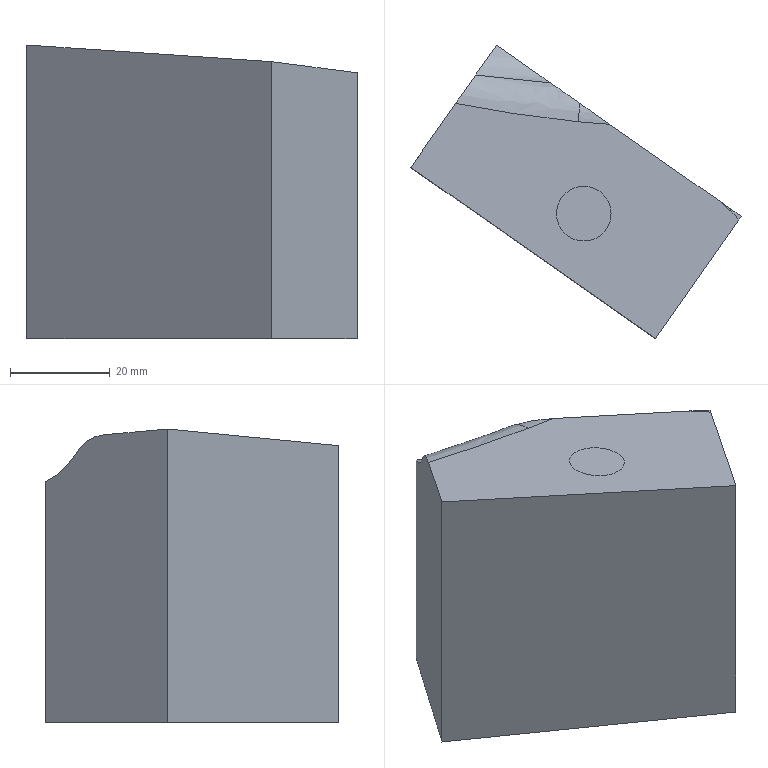Part | NX | features solid 2 | 1 solid | 12 faces | box 66.356 x 58.989 x 59.079 mm | volume 100854 mm3 | spline 7 | plane 5
STEP:
#1=CARTESIAN_POINT('',(-576.236,51.557,-40.));
#2=VERTEX_POINT('',#1);
#3=CARTESIAN_POINT('',(-559.029,76.131,-40.));
#4=VERTEX_POINT('',#3);
#5=CARTESIAN_POINT('',(-576.236,51.557,-40.));
#6=DIRECTION('',(-0.5736,-0.8192,0.));
#7=VECTOR('',#6,1000.);
#8=LINE('',#5,#7);
#9=EDGE_CURVE('',#2,#4,#8,.F.);
#10=ORIENTED_EDGE('',*,*,#9,.F.);
#11=CARTESIAN_POINT('',(-625.385,85.971,-40.));
#12=VERTEX_POINT('',#11);
#13=CARTESIAN_POINT('',(-543.47,28.614,-40.));
#14=DIRECTION('',(-0.8192,0.5736,0.));
#15=VECTOR('',#14,1000.);
#16=LINE('',#13,#15);
#17=EDGE_CURVE('',#12,#2,#16,.F.);
#18=ORIENTED_EDGE('',*,*,#17,.F.);
#19=CARTESIAN_POINT('',(-608.178,110.546,-40.));
#20=VERTEX_POINT('',#19);
#21=CARTESIAN_POINT('',(-625.385,85.971,-40.));
#22=DIRECTION('',(-0.5736,-0.8192,0.));
#23=VECTOR('',#22,1000.);
#24=LINE('',#21,#23);
#25=EDGE_CURVE('',#12,#20,#24,.F.);
#26=ORIENTED_EDGE('',*,*,#25,.T.);
#27=CARTESIAN_POINT('',(-526.263,53.188,-40.));
#28=DIRECTION('',(-0.8192,0.5736,0.));
#29=VECTOR('',#28,1000.);
#30=LINE('',#27,#29);
#31=EDGE_CURVE('',#20,#4,#30,.F.);
#32=ORIENTED_EDGE('',*,*,#31,.T.);
#33=EDGE_LOOP('',(#10,#18,#26,#32));
#34=FACE_BOUND('',#33,.T.);
#35=CARTESIAN_POINT('',(-543.47,28.614,-40.));
#36=DIRECTION('',(0.,0.,1.));
#37=DIRECTION('',(-0.8192,0.5736,0.));
#38=AXIS2_PLACEMENT_3D('',#35,#36,#37);
#39=PLANE('',#38);
#40=ADVANCED_FACE('',(#34),#39,.F.);
#41=CARTESIAN_POINT('',(-563.258,79.093,13.789));
#42=VERTEX_POINT('',#41);
#43=CARTESIAN_POINT('',(-560.662,77.274,13.604));
#44=VERTEX_POINT('',#43);
#45=CARTESIAN_POINT('',(-563.258,79.093,13.789));
#46=CARTESIAN_POINT('',(-562.393,78.487,13.731));
#47=CARTESIAN_POINT('',(-561.527,77.88,13.669));
#48=CARTESIAN_POINT('',(-560.661,77.274,13.604));
#49=B_SPLINE_CURVE_WITH_KNOTS('',3,(#45,#46,#47,#48),.UNSPECIFIED.,.F.,.F.,(4,4),(0.,0.003176),.UNSPECIFIED.);
#50=EDGE_CURVE('',#42,#44,#49,.T.);
#51=ORIENTED_EDGE('',*,*,#50,.T.);
#52=CARTESIAN_POINT('',(-559.029,76.131,13.461));
#53=VERTEX_POINT('',#52);
#54=CARTESIAN_POINT('',(-560.662,77.275,13.604));
#55=CARTESIAN_POINT('',(-560.117,76.893,13.563));
#56=CARTESIAN_POINT('',(-559.573,76.512,13.519));
#57=CARTESIAN_POINT('',(-559.029,76.131,13.461));
#58=B_SPLINE_CURVE_WITH_KNOTS('',3,(#54,#55,#56,#57),.UNSPECIFIED.,.F.,.F.,(4,4),(0.0004081,0.002407),.UNSPECIFIED.);
#59=EDGE_CURVE('',#44,#53,#58,.T.);
#60=ORIENTED_EDGE('',*,*,#59,.T.);
#61=CARTESIAN_POINT('',(-559.029,76.131,80.));
#62=DIRECTION('',(0.,0.,-1.));
#63=VECTOR('',#62,1000.);
#64=LINE('',#61,#63);
#65=EDGE_CURVE('',#53,#4,#64,.T.);
#66=ORIENTED_EDGE('',*,*,#65,.T.);
#67=ORIENTED_EDGE('',*,*,#31,.F.);
#68=CARTESIAN_POINT('',(-608.178,110.546,8.511));
#69=VERTEX_POINT('',#68);
#70=CARTESIAN_POINT('',(-608.178,110.546,80.));
#71=DIRECTION('',(0.,0.,-1.));
#72=VECTOR('',#71,1000.);
#73=LINE('',#70,#72);
#74=EDGE_CURVE('',#69,#20,#73,.T.);
#75=ORIENTED_EDGE('',*,*,#74,.F.);
#76=CARTESIAN_POINT('',(-597.294,102.925,11.329));
#77=VERTEX_POINT('',#76);
#78=CARTESIAN_POINT('',(-608.178,110.546,8.511));
#79=CARTESIAN_POINT('',(-606.271,109.211,8.19));
#80=CARTESIAN_POINT('',(-603.392,107.195,8.072));
#81=CARTESIAN_POINT('',(-599.628,104.559,9.191));
#82=CARTESIAN_POINT('',(-597.942,103.379,10.457));
#83=CARTESIAN_POINT('',(-597.295,102.925,11.328));
#84=B_SPLINE_CURVE_WITH_KNOTS('',3,(#78,#79,#80,#81,#82,#83),.UNSPECIFIED.,.F.,.F.,(4,1,1,4),(0.,0.006983,0.01047,0.01397),.UNSPECIFIED.);
#85=EDGE_CURVE('',#69,#77,#84,.T.);
#86=ORIENTED_EDGE('',*,*,#85,.T.);
#87=CARTESIAN_POINT('',(-591.493,98.863,14.745));
#88=VERTEX_POINT('',#87);
#89=CARTESIAN_POINT('',(-597.294,102.924,11.33));
#90=CARTESIAN_POINT('',(-596.55,102.404,12.332));
#91=CARTESIAN_POINT('',(-594.649,101.073,13.706));
#92=CARTESIAN_POINT('',(-592.562,99.612,14.469));
#93=CARTESIAN_POINT('',(-591.492,98.862,14.745));
#94=B_SPLINE_CURVE_WITH_KNOTS('',3,(#89,#90,#91,#92,#93),.UNSPECIFIED.,.F.,.F.,(4,1,4),(0.,0.00397,0.007939),.UNSPECIFIED.);
#95=EDGE_CURVE('',#77,#88,#94,.T.);
#96=ORIENTED_EDGE('',*,*,#95,.T.);
#97=CARTESIAN_POINT('',(-585.405,94.6,15.297));
#98=VERTEX_POINT('',#97);
#99=CARTESIAN_POINT('',(-585.405,94.6,15.296));
#100=CARTESIAN_POINT('',(-586.428,95.316,15.367));
#101=CARTESIAN_POINT('',(-588.482,96.754,15.411));
#102=CARTESIAN_POINT('',(-590.493,98.163,15.003));
#103=CARTESIAN_POINT('',(-591.495,98.864,14.744));
#104=B_SPLINE_CURVE_WITH_KNOTS('',3,(#99,#100,#101,#102,#103),.UNSPECIFIED.,.F.,.F.,(4,1,4),(0.004974,0.008726,0.01248),.UNSPECIFIED.);
#105=EDGE_CURVE('',#98,#88,#104,.T.);
#106=ORIENTED_EDGE('',*,*,#105,.F.);
#107=CARTESIAN_POINT('',(-611.053,112.559,17.042));
#108=DIRECTION('',(-0.8179,0.5727,0.05566));
#109=VECTOR('',#108,1000.);
#110=LINE('',#107,#109);
#111=EDGE_CURVE('',#98,#42,#110,.F.);
#112=ORIENTED_EDGE('',*,*,#111,.T.);
#113=EDGE_LOOP('',(#51,#60,#66,#67,#75,#86,#96,#106,#112));
#114=FACE_BOUND('',#113,.T.);
#115=CARTESIAN_POINT('',(-608.178,110.546,80.));
#116=DIRECTION('',(0.5736,0.8192,0.));
#117=DIRECTION('',(-0.8192,0.5736,0.));
#118=AXIS2_PLACEMENT_3D('',#115,#116,#117);
#119=PLANE('',#118);
#120=ADVANCED_FACE('',(#114),#119,.T.);
#121=CARTESIAN_POINT('',(-625.385,85.971,19.079));
#122=VERTEX_POINT('',#121);
#123=CARTESIAN_POINT('',(-625.385,85.971,80.));
#124=DIRECTION('',(0.,0.,-1.));
#125=VECTOR('',#124,1000.);
#126=LINE('',#123,#125);
#127=EDGE_CURVE('',#122,#12,#126,.T.);
#128=ORIENTED_EDGE('',*,*,#127,.F.);
#129=CARTESIAN_POINT('',(-616.399,98.804,17.913));
#130=VERTEX_POINT('',#129);
#131=CARTESIAN_POINT('',(-627.971,82.279,19.414));
#132=DIRECTION('',(-0.572,-0.8169,0.0742));
#133=VECTOR('',#132,1000.);
#134=LINE('',#131,#133);
#135=EDGE_CURVE('',#122,#130,#134,.F.);
#136=ORIENTED_EDGE('',*,*,#135,.T.);
#137=CARTESIAN_POINT('',(-612.406,104.507,14.025));
#138=VERTEX_POINT('',#137);
#139=CARTESIAN_POINT('',(-616.399,98.805,17.913));
#140=CARTESIAN_POINT('',(-614.817,101.064,17.708));
#141=CARTESIAN_POINT('',(-613.314,103.21,16.305));
#142=CARTESIAN_POINT('',(-612.408,104.504,14.03));
#143=B_SPLINE_CURVE_WITH_KNOTS('',3,(#139,#140,#141,#142),.UNSPECIFIED.,.F.,.F.,(4,4),(0.,0.008252),.UNSPECIFIED.);
#144=EDGE_CURVE('',#130,#138,#143,.T.);
#145=ORIENTED_EDGE('',*,*,#144,.T.);
#146=CARTESIAN_POINT('',(-612.406,104.508,14.024));
#147=CARTESIAN_POINT('',(-611.379,105.974,11.449));
#148=CARTESIAN_POINT('',(-609.88,108.114,9.542));
#149=CARTESIAN_POINT('',(-608.178,110.546,8.511));
#150=B_SPLINE_CURVE_WITH_KNOTS('',3,(#146,#147,#148,#149),.UNSPECIFIED.,.F.,.F.,(4,4),(0.003915,0.01322),.UNSPECIFIED.);
#151=EDGE_CURVE('',#138,#69,#150,.T.);
#152=ORIENTED_EDGE('',*,*,#151,.T.);
#153=ORIENTED_EDGE('',*,*,#74,.T.);
#154=ORIENTED_EDGE('',*,*,#25,.F.);
#155=EDGE_LOOP('',(#128,#136,#145,#152,#153,#154));
#156=FACE_BOUND('',#155,.T.);
#157=CARTESIAN_POINT('',(-625.385,85.971,80.));
#158=DIRECTION('',(-0.8192,0.5736,0.));
#159=DIRECTION('',(-0.5736,-0.8192,0.));
#160=AXIS2_PLACEMENT_3D('',#157,#158,#159);
#161=PLANE('',#160);
#162=ADVANCED_FACE('',(#156),#161,.T.);
#163=CARTESIAN_POINT('',(-576.236,51.557,15.734));
#164=VERTEX_POINT('',#163);
#165=CARTESIAN_POINT('',(-628.159,87.913,19.267));
#166=DIRECTION('',(-0.8179,0.5727,0.05566));
#167=VECTOR('',#166,1000.);
#168=LINE('',#165,#167);
#169=EDGE_CURVE('',#122,#164,#168,.F.);
#170=ORIENTED_EDGE('',*,*,#169,.F.);
#171=ORIENTED_EDGE('',*,*,#127,.T.);
#172=ORIENTED_EDGE('',*,*,#17,.T.);
#173=CARTESIAN_POINT('',(-576.236,51.557,80.));
#174=DIRECTION('',(0.,0.,-1.));
#175=VECTOR('',#174,1000.);
#176=LINE('',#173,#175);
#177=EDGE_CURVE('',#164,#2,#176,.T.);
#178=ORIENTED_EDGE('',*,*,#177,.F.);
#179=EDGE_LOOP('',(#170,#171,#172,#178));
#180=FACE_BOUND('',#179,.T.);
#181=CARTESIAN_POINT('',(-625.385,85.971,80.));
#182=DIRECTION('',(0.5736,0.8192,0.));
#183=DIRECTION('',(-0.8192,0.5736,0.));
#184=AXIS2_PLACEMENT_3D('',#181,#182,#183);
#185=PLANE('',#184);
#186=ADVANCED_FACE('',(#180),#185,.F.);
#187=CARTESIAN_POINT('',(-559.56,75.373,13.571));
#188=VERTEX_POINT('',#187);
#189=CARTESIAN_POINT('',(-578.964,47.661,16.088));
#190=DIRECTION('',(-0.572,-0.8169,0.0742));
#191=VECTOR('',#190,1000.);
#192=LINE('',#189,#191);
#193=EDGE_CURVE('',#164,#188,#192,.F.);
#194=ORIENTED_EDGE('',*,*,#193,.F.);
#195=ORIENTED_EDGE('',*,*,#177,.T.);
#196=ORIENTED_EDGE('',*,*,#9,.T.);
#197=ORIENTED_EDGE('',*,*,#65,.F.);
#198=CARTESIAN_POINT('',(-559.56,75.373,13.57));
#199=CARTESIAN_POINT('',(-559.383,75.626,13.547));
#200=CARTESIAN_POINT('',(-559.206,75.879,13.512));
#201=CARTESIAN_POINT('',(-559.029,76.131,13.461));
#202=B_SPLINE_CURVE_WITH_KNOTS('',3,(#198,#199,#200,#201),.UNSPECIFIED.,.F.,.F.,(4,4),(0.003283,0.004211),.UNSPECIFIED.);
#203=EDGE_CURVE('',#188,#53,#202,.T.);
#204=ORIENTED_EDGE('',*,*,#203,.F.);
#205=EDGE_LOOP('',(#194,#195,#196,#197,#204));
#206=FACE_BOUND('',#205,.T.);
#207=CARTESIAN_POINT('',(-576.236,51.557,80.));
#208=DIRECTION('',(-0.8192,0.5736,0.));
#209=DIRECTION('',(-0.5736,-0.8192,0.));
#210=AXIS2_PLACEMENT_3D('',#207,#208,#209);
#211=PLANE('',#210);
#212=ADVANCED_FACE('',(#206),#211,.F.);
#213=CARTESIAN_POINT('',(-596.124,76.649,16.764));
#214=VERTEX_POINT('',#213);
#215=CARTESIAN_POINT('',(-585.166,76.649,15.796));
#216=VERTEX_POINT('',#215);
#217=CARTESIAN_POINT('',(-596.124,76.649,16.764));
#218=CARTESIAN_POINT('',(-596.122,75.89,16.785));
#219=CARTESIAN_POINT('',(-595.863,74.494,16.803));
#220=CARTESIAN_POINT('',(-594.599,72.667,16.744));
#221=CARTESIAN_POINT('',(-592.796,71.409,16.621));
#222=CARTESIAN_POINT('',(-590.631,71.023,16.441));
#223=CARTESIAN_POINT('',(-588.469,71.408,16.239));
#224=CARTESIAN_POINT('',(-586.671,72.667,16.044));
#225=CARTESIAN_POINT('',(-585.416,74.494,15.88));
#226=CARTESIAN_POINT('',(-585.165,75.89,15.818));
#227=CARTESIAN_POINT('',(-585.166,76.649,15.796));
#228=B_SPLINE_CURVE_WITH_KNOTS('',3,(#217,#218,#219,#220,#221,#222,#223,#224,#225,#226,#227),.UNSPECIFIED.,.F.,.F.,(4,1,1,1,1,1,1,1,4),(0.,0.125,0.25,0.375,0.5,0.625,0.75,0.875,1.),.UNSPECIFIED.);
#229=EDGE_CURVE('',#214,#216,#228,.T.);
#230=ORIENTED_EDGE('',*,*,#229,.F.);
#231=CARTESIAN_POINT('',(-585.166,76.649,15.796));
#232=CARTESIAN_POINT('',(-585.168,77.408,15.774));
#233=CARTESIAN_POINT('',(-585.427,78.804,15.756));
#234=CARTESIAN_POINT('',(-586.691,80.632,15.815));
#235=CARTESIAN_POINT('',(-588.494,81.89,15.938));
#236=CARTESIAN_POINT('',(-590.66,82.275,16.118));
#237=CARTESIAN_POINT('',(-592.822,81.89,16.32));
#238=CARTESIAN_POINT('',(-594.62,80.631,16.515));
#239=CARTESIAN_POINT('',(-595.874,78.804,16.679));
#240=CARTESIAN_POINT('',(-596.126,77.408,16.742));
#241=CARTESIAN_POINT('',(-596.124,76.649,16.764));
#242=B_SPLINE_CURVE_WITH_KNOTS('',3,(#231,#232,#233,#234,#235,#236,#237,#238,#239,#240,#241),.UNSPECIFIED.,.F.,.F.,(4,1,1,1,1,1,1,1,4),(0.,0.125,0.25,0.375,0.5,0.625,0.75,0.875,1.),.UNSPECIFIED.);
#243=EDGE_CURVE('',#216,#214,#242,.T.);
#244=ORIENTED_EDGE('',*,*,#243,.F.);
#245=EDGE_LOOP('',(#230,#244));
#246=FACE_BOUND('',#245,.T.);
#247=ORIENTED_EDGE('',*,*,#193,.T.);
#248=CARTESIAN_POINT('',(-560.907,76.996,13.642));
#249=VERTEX_POINT('',#248);
#250=CARTESIAN_POINT('',(-560.907,76.996,13.643));
#251=CARTESIAN_POINT('',(-560.377,76.523,13.609));
#252=CARTESIAN_POINT('',(-559.928,75.982,13.585));
#253=CARTESIAN_POINT('',(-559.56,75.373,13.571));
#254=B_SPLINE_CURVE_WITH_KNOTS('',3,(#250,#251,#252,#253),.UNSPECIFIED.,.F.,.F.,(4,4),(0.,0.1448),.UNSPECIFIED.);
#255=EDGE_CURVE('',#249,#188,#254,.T.);
#256=ORIENTED_EDGE('',*,*,#255,.F.);
#257=CARTESIAN_POINT('',(-563.258,79.093,13.789));
#258=CARTESIAN_POINT('',(-562.475,78.394,13.741));
#259=CARTESIAN_POINT('',(-561.691,77.695,13.692));
#260=CARTESIAN_POINT('',(-560.907,76.996,13.643));
#261=B_SPLINE_CURVE_WITH_KNOTS('',3,(#257,#258,#259,#260),.UNSPECIFIED.,.F.,.F.,(4,4),(0.7162,1.),.UNSPECIFIED.);
#262=EDGE_CURVE('',#42,#249,#261,.T.);
#263=ORIENTED_EDGE('',*,*,#262,.F.);
#264=ORIENTED_EDGE('',*,*,#111,.F.);
#265=CARTESIAN_POINT('',(-591.763,95.106,15.844));
#266=VERTEX_POINT('',#265);
#267=CARTESIAN_POINT('',(-591.763,95.106,15.844));
#268=CARTESIAN_POINT('',(-591.046,95.028,15.783));
#269=CARTESIAN_POINT('',(-589.684,94.91,15.666));
#270=CARTESIAN_POINT('',(-586.956,94.733,15.43));
#271=CARTESIAN_POINT('',(-585.872,94.643,15.337));
#272=CARTESIAN_POINT('',(-585.405,94.6,15.297));
#273=B_SPLINE_CURVE_WITH_KNOTS('',3,(#267,#268,#269,#270,#271,#272),.UNSPECIFIED.,.F.,.F.,(4,1,1,4),(0.,0.2009,0.3013,0.4018),.UNSPECIFIED.);
#274=EDGE_CURVE('',#266,#98,#273,.T.);
#275=ORIENTED_EDGE('',*,*,#274,.F.);
#276=CARTESIAN_POINT('',(-616.4,98.803,17.913));
#277=CARTESIAN_POINT('',(-609.032,97.318,17.305));
#278=CARTESIAN_POINT('',(-600.82,96.086,16.615));
#279=CARTESIAN_POINT('',(-591.763,95.106,15.844));
#280=B_SPLINE_CURVE_WITH_KNOTS('',3,(#276,#277,#278,#279),.UNSPECIFIED.,.F.,.F.,(4,4),(0.5958,1.),.UNSPECIFIED.);
#281=EDGE_CURVE('',#130,#266,#280,.T.);
#282=ORIENTED_EDGE('',*,*,#281,.F.);
#283=ORIENTED_EDGE('',*,*,#135,.F.);
#284=ORIENTED_EDGE('',*,*,#169,.T.);
#285=EDGE_LOOP('',(#247,#256,#263,#264,#275,#282,#283,#284));
#286=FACE_BOUND('',#285,.T.);
#287=CARTESIAN_POINT('',(-559.104,51.273,14.228));
#288=CARTESIAN_POINT('',(-559.225,99.087,12.854));
#289=CARTESIAN_POINT('',(-625.692,51.273,20.111));
#290=CARTESIAN_POINT('',(-625.813,99.087,18.736));
#291=B_SPLINE_SURFACE_WITH_KNOTS('',1,1,((#287,#288),(#289,#290)),.PLANE_SURF.,.F.,.F.,.F.,(2,2),(2,2),(0.1376,0.7683),(0.09843,0.4027),.PIECEWISE_BEZIER_KNOTS.);
#292=ADVANCED_FACE('',(#246,#286),#291,.F.);
#293=ORIENTED_EDGE('',*,*,#203,.T.);
#294=ORIENTED_EDGE('',*,*,#59,.F.);
#295=CARTESIAN_POINT('',(-560.662,77.275,13.604));
#296=CARTESIAN_POINT('',(-560.743,77.182,13.619));
#297=CARTESIAN_POINT('',(-560.824,77.09,13.632));
#298=CARTESIAN_POINT('',(-560.907,76.996,13.642));
#299=B_SPLINE_CURVE_WITH_KNOTS('',3,(#295,#296,#297,#298),.UNSPECIFIED.,.F.,.F.,(4,4),(0.9245,1.),.UNSPECIFIED.);
#300=EDGE_CURVE('',#44,#249,#299,.T.);
#301=ORIENTED_EDGE('',*,*,#300,.T.);
#302=ORIENTED_EDGE('',*,*,#255,.T.);
#303=EDGE_LOOP('',(#293,#294,#301,#302));
#304=FACE_BOUND('',#303,.T.);
#305=CARTESIAN_POINT('',(-559.029,75.361,13.513));
#306=CARTESIAN_POINT('',(-559.043,75.361,13.515));
#307=CARTESIAN_POINT('',(-559.058,75.361,13.517));
#308=CARTESIAN_POINT('',(-559.073,75.361,13.519));
#309=CARTESIAN_POINT('',(-559.457,75.362,13.566));
#310=CARTESIAN_POINT('',(-559.852,75.361,13.601));
#311=CARTESIAN_POINT('',(-560.243,75.359,13.623));
#312=CARTESIAN_POINT('',(-560.644,75.356,13.634));
#313=CARTESIAN_POINT('',(-561.055,75.352,13.634));
#314=CARTESIAN_POINT('',(-559.027,75.439,13.509));
#315=CARTESIAN_POINT('',(-559.041,75.439,13.511));
#316=CARTESIAN_POINT('',(-559.056,75.439,13.513));
#317=CARTESIAN_POINT('',(-559.071,75.439,13.515));
#318=CARTESIAN_POINT('',(-559.454,75.44,13.564));
#319=CARTESIAN_POINT('',(-559.848,75.439,13.6));
#320=CARTESIAN_POINT('',(-560.238,75.438,13.623));
#321=CARTESIAN_POINT('',(-560.637,75.435,13.635));
#322=CARTESIAN_POINT('',(-561.047,75.431,13.637));
#323=CARTESIAN_POINT('',(-559.025,75.517,13.504));
#324=CARTESIAN_POINT('',(-559.039,75.517,13.506));
#325=CARTESIAN_POINT('',(-559.054,75.517,13.508));
#326=CARTESIAN_POINT('',(-559.069,75.517,13.51));
#327=CARTESIAN_POINT('',(-559.45,75.518,13.56));
#328=CARTESIAN_POINT('',(-559.843,75.518,13.598));
#329=CARTESIAN_POINT('',(-560.232,75.516,13.622));
#330=CARTESIAN_POINT('',(-560.63,75.514,13.636));
#331=CARTESIAN_POINT('',(-561.039,75.51,13.639));
#332=CARTESIAN_POINT('',(-559.023,75.595,13.5));
#333=CARTESIAN_POINT('',(-559.038,75.595,13.502));
#334=CARTESIAN_POINT('',(-559.052,75.595,13.504));
#335=CARTESIAN_POINT('',(-559.067,75.595,13.506));
#336=CARTESIAN_POINT('',(-559.447,75.596,13.557));
#337=CARTESIAN_POINT('',(-559.839,75.596,13.596));
#338=CARTESIAN_POINT('',(-560.227,75.595,13.621));
#339=CARTESIAN_POINT('',(-560.624,75.592,13.636));
#340=CARTESIAN_POINT('',(-561.031,75.588,13.641));
#341=CARTESIAN_POINT('',(-559.016,75.979,13.474));
#342=CARTESIAN_POINT('',(-559.031,75.979,13.477));
#343=CARTESIAN_POINT('',(-559.045,75.979,13.479));
#344=CARTESIAN_POINT('',(-559.06,75.979,13.481));
#345=CARTESIAN_POINT('',(-559.434,75.981,13.539));
#346=CARTESIAN_POINT('',(-559.82,75.982,13.584));
#347=CARTESIAN_POINT('',(-560.201,75.981,13.617));
#348=CARTESIAN_POINT('',(-560.592,75.979,13.639));
#349=CARTESIAN_POINT('',(-560.992,75.976,13.65));
#350=CARTESIAN_POINT('',(-559.016,76.362,13.442));
#351=CARTESIAN_POINT('',(-559.03,76.363,13.445));
#352=CARTESIAN_POINT('',(-559.044,76.363,13.447));
#353=CARTESIAN_POINT('',(-559.059,76.363,13.45));
#354=CARTESIAN_POINT('',(-559.427,76.365,13.514));
#355=CARTESIAN_POINT('',(-559.806,76.367,13.567));
#356=CARTESIAN_POINT('',(-560.18,76.367,13.607));
#357=CARTESIAN_POINT('',(-560.564,76.366,13.636));
#358=CARTESIAN_POINT('',(-560.956,76.364,13.656));
#359=CARTESIAN_POINT('',(-559.021,76.667,13.41));
#360=CARTESIAN_POINT('',(-559.035,76.668,13.413));
#361=CARTESIAN_POINT('',(-559.049,76.668,13.416));
#362=CARTESIAN_POINT('',(-559.063,76.668,13.418));
#363=CARTESIAN_POINT('',(-559.427,76.671,13.488));
#364=CARTESIAN_POINT('',(-559.801,76.673,13.546));
#365=CARTESIAN_POINT('',(-560.169,76.674,13.593));
#366=CARTESIAN_POINT('',(-560.547,76.673,13.629));
#367=CARTESIAN_POINT('',(-560.933,76.672,13.655));
#368=CARTESIAN_POINT('',(-559.033,76.972,13.372));
#369=CARTESIAN_POINT('',(-559.047,76.972,13.375));
#370=CARTESIAN_POINT('',(-559.061,76.972,13.377));
#371=CARTESIAN_POINT('',(-559.074,76.972,13.38));
#372=CARTESIAN_POINT('',(-559.433,76.976,13.455));
#373=CARTESIAN_POINT('',(-559.802,76.978,13.519));
#374=CARTESIAN_POINT('',(-560.165,76.98,13.571));
#375=CARTESIAN_POINT('',(-560.536,76.98,13.614));
#376=CARTESIAN_POINT('',(-560.917,76.98,13.647));
#377=CARTESIAN_POINT('',(-559.051,77.275,13.326));
#378=CARTESIAN_POINT('',(-559.064,77.276,13.329));
#379=CARTESIAN_POINT('',(-559.078,77.276,13.333));
#380=CARTESIAN_POINT('',(-559.092,77.276,13.336));
#381=CARTESIAN_POINT('',(-559.446,77.28,13.415));
#382=CARTESIAN_POINT('',(-559.809,77.283,13.485));
#383=CARTESIAN_POINT('',(-560.167,77.285,13.543));
#384=CARTESIAN_POINT('',(-560.533,77.286,13.591));
#385=CARTESIAN_POINT('',(-560.908,77.286,13.631));
#386=B_SPLINE_SURFACE_WITH_KNOTS('',5,5,((#305,#306,#307,#308,#309,#310,#311,#312,#313),(#314,#315,#316,#317,#318,#319,#320,#321,#322),(#323,#324,#325,#326,#327,#328,#329,#330,#331),(#332,#333,#334,#335,#336,#337,#338,#339,#340),(#341,#342,#343,#344,#345,#346,#347,#348,#349),(#350,#351,#352,#353,#354,#355,#356,#357,#358),(#359,#360,#361,#362,#363,#364,#365,#366,#367),(#368,#369,#370,#371,#372,#373,#374,#375,#376),(#377,#378,#379,#380,#381,#382,#383,#384,#385)),.UNSPECIFIED.,.F.,.F.,.F.,(6,3,6),(6,3,6),(0.65,0.6694,0.7453),(0.885,0.8892,0.9947),.UNSPECIFIED.);
#387=ADVANCED_FACE('',(#304),#386,.T.);
#388=CARTESIAN_POINT('',(-597.294,102.925,11.328));
#389=CARTESIAN_POINT('',(-603.16,103.448,12.375));
#390=CARTESIAN_POINT('',(-608.198,103.994,13.271));
#391=CARTESIAN_POINT('',(-612.407,104.508,14.024));
#392=B_SPLINE_CURVE_WITH_KNOTS('',3,(#388,#389,#390,#391),.UNSPECIFIED.,.F.,.F.,(4,4),(0.07589,0.3184),.UNSPECIFIED.);
#393=EDGE_CURVE('',#138,#77,#392,.F.);
#394=ORIENTED_EDGE('',*,*,#393,.T.);
#395=ORIENTED_EDGE('',*,*,#85,.F.);
#396=ORIENTED_EDGE('',*,*,#151,.F.);
#397=EDGE_LOOP('',(#394,#395,#396));
#398=FACE_BOUND('',#397,.T.);
#399=CARTESIAN_POINT('',(-598.658,110.234,5.604));
#400=CARTESIAN_POINT('',(-613.453,110.804,10.105));
#401=CARTESIAN_POINT('',(-598.591,106.877,6.251));
#402=CARTESIAN_POINT('',(-613.385,107.448,10.753));
#403=CARTESIAN_POINT('',(-598.059,104.227,8.336));
#404=CARTESIAN_POINT('',(-612.853,104.798,12.837));
#405=CARTESIAN_POINT('',(-597.193,102.9,11.351));
#406=CARTESIAN_POINT('',(-611.987,103.471,15.852));
#407=(BOUNDED_SURFACE()B_SPLINE_SURFACE(3,1,((#399,#400),(#401,#402),(#403,#404),(#405,#406)),.CYLINDRICAL_SURF.,.F.,.F.,.F.)B_SPLINE_SURFACE_WITH_KNOTS((4,4),(2,2),(0.139,0.8942),(0.4904,0.6463),.PIECEWISE_BEZIER_KNOTS.)GEOMETRIC_REPRESENTATION_ITEM()RATIONAL_B_SPLINE_SURFACE(((0.9525,0.9525),(0.8804,0.8804),(0.8837,0.8837),(0.9625,0.9625)))REPRESENTATION_ITEM('')SURFACE());
#408=ADVANCED_FACE('',(#398),#407,.F.);
#409=ORIENTED_EDGE('',*,*,#281,.T.);
#410=CARTESIAN_POINT('',(-591.492,98.863,14.744));
#411=CARTESIAN_POINT('',(-591.545,97.725,15.413));
#412=CARTESIAN_POINT('',(-591.639,96.421,15.795));
#413=CARTESIAN_POINT('',(-591.763,95.106,15.844));
#414=B_SPLINE_CURVE_WITH_KNOTS('',3,(#410,#411,#412,#413),.UNSPECIFIED.,.F.,.F.,(4,4),(0.5957,1.),.UNSPECIFIED.);
#415=EDGE_CURVE('',#266,#88,#414,.F.);
#416=ORIENTED_EDGE('',*,*,#415,.T.);
#417=ORIENTED_EDGE('',*,*,#95,.F.);
#418=ORIENTED_EDGE('',*,*,#393,.F.);
#419=ORIENTED_EDGE('',*,*,#144,.F.);
#420=EDGE_LOOP('',(#409,#416,#417,#418,#419));
#421=FACE_BOUND('',#420,.T.);
#422=CARTESIAN_POINT('',(-591.763,95.106,15.844));
#423=CARTESIAN_POINT('',(-591.661,96.081,15.806));
#424=CARTESIAN_POINT('',(-591.572,97.051,15.619));
#425=CARTESIAN_POINT('',(-591.499,97.987,15.284));
#426=CARTESIAN_POINT('',(-591.391,99.728,14.337));
#427=CARTESIAN_POINT('',(-591.363,101.112,12.913));
#428=CARTESIAN_POINT('',(-591.37,101.689,12.101));
#429=CARTESIAN_POINT('',(-591.397,102.134,11.214));
#430=CARTESIAN_POINT('',(-591.444,102.436,10.282));
#431=CARTESIAN_POINT('',(-595.835,95.546,16.191));
#432=CARTESIAN_POINT('',(-595.725,96.481,16.154));
#433=CARTESIAN_POINT('',(-595.628,97.412,15.979));
#434=CARTESIAN_POINT('',(-595.546,98.312,15.668));
#435=CARTESIAN_POINT('',(-595.417,99.997,14.79));
#436=CARTESIAN_POINT('',(-595.365,101.365,13.465));
#437=CARTESIAN_POINT('',(-595.359,101.948,12.706));
#438=CARTESIAN_POINT('',(-595.375,102.411,11.874));
#439=CARTESIAN_POINT('',(-595.409,102.747,10.993));
#440=CARTESIAN_POINT('',(-599.898,96.047,16.535));
#441=CARTESIAN_POINT('',(-599.782,96.94,16.499));
#442=CARTESIAN_POINT('',(-599.677,97.831,16.337));
#443=CARTESIAN_POINT('',(-599.586,98.694,16.049));
#444=CARTESIAN_POINT('',(-599.437,100.319,15.238));
#445=CARTESIAN_POINT('',(-599.362,101.665,14.011));
#446=CARTESIAN_POINT('',(-599.344,102.249,13.306));
#447=CARTESIAN_POINT('',(-599.346,102.727,12.53));
#448=CARTESIAN_POINT('',(-599.368,103.09,11.702));
#449=CARTESIAN_POINT('',(-603.953,96.611,16.877));
#450=CARTESIAN_POINT('',(-603.83,97.463,16.841));
#451=CARTESIAN_POINT('',(-603.717,98.311,16.691));
#452=CARTESIAN_POINT('',(-603.618,99.136,16.426));
#453=CARTESIAN_POINT('',(-603.45,100.697,15.682));
#454=CARTESIAN_POINT('',(-603.351,102.015,14.551));
#455=CARTESIAN_POINT('',(-603.321,102.595,13.901));
#456=CARTESIAN_POINT('',(-603.31,103.083,13.18));
#457=CARTESIAN_POINT('',(-603.319,103.47,12.409));
#458=CARTESIAN_POINT('',(-608.911,97.392,17.292));
#459=CARTESIAN_POINT('',(-608.781,98.19,17.258));
#460=CARTESIAN_POINT('',(-608.66,98.985,17.122));
#461=CARTESIAN_POINT('',(-608.55,99.76,16.885));
#462=CARTESIAN_POINT('',(-608.36,101.238,16.22));
#463=CARTESIAN_POINT('',(-608.233,102.511,15.207));
#464=CARTESIAN_POINT('',(-608.187,103.083,14.623));
#465=CARTESIAN_POINT('',(-608.16,103.576,13.973));
#466=CARTESIAN_POINT('',(-608.151,103.983,13.272));
#467=CARTESIAN_POINT('',(-613.852,98.306,17.702));
#468=CARTESIAN_POINT('',(-613.715,99.047,17.669));
#469=CARTESIAN_POINT('',(-613.586,99.786,17.547));
#470=CARTESIAN_POINT('',(-613.468,100.508,17.337));
#471=CARTESIAN_POINT('',(-613.256,101.892,16.749));
#472=CARTESIAN_POINT('',(-613.101,103.109,15.854));
#473=CARTESIAN_POINT('',(-613.039,103.663,15.336));
#474=CARTESIAN_POINT('',(-612.995,104.153,14.757));
#475=CARTESIAN_POINT('',(-612.968,104.571,14.13));
#476=CARTESIAN_POINT('',(-614.751,98.478,17.777));
#477=CARTESIAN_POINT('',(-614.613,99.208,17.743));
#478=CARTESIAN_POINT('',(-614.483,99.936,17.624));
#479=CARTESIAN_POINT('',(-614.362,100.648,17.419));
#480=CARTESIAN_POINT('',(-614.147,102.015,16.846));
#481=CARTESIAN_POINT('',(-613.987,103.221,15.971));
#482=CARTESIAN_POINT('',(-613.922,103.772,15.465));
#483=CARTESIAN_POINT('',(-613.875,104.261,14.9));
#484=CARTESIAN_POINT('',(-613.845,104.681,14.286));
#485=CARTESIAN_POINT('',(-615.649,98.654,17.851));
#486=CARTESIAN_POINT('',(-615.51,99.373,17.818));
#487=CARTESIAN_POINT('',(-615.378,100.091,17.701));
#488=CARTESIAN_POINT('',(-615.256,100.793,17.501));
#489=CARTESIAN_POINT('',(-615.037,102.142,16.942));
#490=CARTESIAN_POINT('',(-614.872,103.337,16.088));
#491=CARTESIAN_POINT('',(-614.804,103.884,15.595));
#492=CARTESIAN_POINT('',(-614.754,104.372,15.042));
#493=CARTESIAN_POINT('',(-614.721,104.793,14.442));
#494=CARTESIAN_POINT('',(-616.546,98.835,17.925));
#495=CARTESIAN_POINT('',(-616.406,99.543,17.892));
#496=CARTESIAN_POINT('',(-616.273,100.25,17.778));
#497=CARTESIAN_POINT('',(-616.149,100.942,17.583));
#498=CARTESIAN_POINT('',(-615.926,102.274,17.037));
#499=CARTESIAN_POINT('',(-615.756,103.456,16.205));
#500=CARTESIAN_POINT('',(-615.686,104.,15.724));
#501=CARTESIAN_POINT('',(-615.632,104.486,15.184));
#502=CARTESIAN_POINT('',(-615.596,104.908,14.598));
#503=B_SPLINE_SURFACE_WITH_KNOTS('',5,5,((#422,#423,#424,#425,#426,#427,#428,#429,#430),(#431,#432,#433,#434,#435,#436,#437,#438,#439),(#440,#441,#442,#443,#444,#445,#446,#447,#448),(#449,#450,#451,#452,#453,#454,#455,#456,#457),(#458,#459,#460,#461,#462,#463,#464,#465,#466),(#467,#468,#469,#470,#471,#472,#473,#474,#475),(#476,#477,#478,#479,#480,#481,#482,#483,#484),(#485,#486,#487,#488,#489,#490,#491,#492,#493),(#494,#495,#496,#497,#498,#499,#500,#501,#502)),.UNSPECIFIED.,.F.,.F.,.F.,(6,3,6),(6,3,6),(0.,0.3404,0.4162),(0.,0.5,1.),.UNSPECIFIED.);
#504=ADVANCED_FACE('',(#421),#503,.F.);
#505=ORIENTED_EDGE('',*,*,#105,.T.);
#506=ORIENTED_EDGE('',*,*,#415,.F.);
#507=ORIENTED_EDGE('',*,*,#274,.T.);
#508=EDGE_LOOP('',(#505,#506,#507));
#509=FACE_BOUND('',#508,.T.);
#510=CARTESIAN_POINT('',(-591.584,98.89,14.742));
#511=CARTESIAN_POINT('',(-591.591,98.563,14.934));
#512=CARTESIAN_POINT('',(-591.601,98.221,15.109));
#513=CARTESIAN_POINT('',(-591.614,97.863,15.266));
#514=CARTESIAN_POINT('',(-591.643,97.25,15.493));
#515=CARTESIAN_POINT('',(-591.685,96.586,15.661));
#516=CARTESIAN_POINT('',(-591.703,96.319,15.717));
#517=CARTESIAN_POINT('',(-591.734,95.892,15.788));
#518=CARTESIAN_POINT('',(-591.772,95.439,15.83));
#519=CARTESIAN_POINT('',(-591.786,95.276,15.841));
#520=CARTESIAN_POINT('',(-591.801,95.11,15.849));
#521=CARTESIAN_POINT('',(-591.817,94.94,15.852));
#522=CARTESIAN_POINT('',(-590.3,98.793,14.605));
#523=CARTESIAN_POINT('',(-590.306,98.468,14.799));
#524=CARTESIAN_POINT('',(-590.316,98.128,14.976));
#525=CARTESIAN_POINT('',(-590.329,97.772,15.136));
#526=CARTESIAN_POINT('',(-590.357,97.164,15.367));
#527=CARTESIAN_POINT('',(-590.397,96.504,15.541));
#528=CARTESIAN_POINT('',(-590.415,96.239,15.599));
#529=CARTESIAN_POINT('',(-590.446,95.813,15.672));
#530=CARTESIAN_POINT('',(-590.483,95.362,15.715));
#531=CARTESIAN_POINT('',(-590.497,95.2,15.727));
#532=CARTESIAN_POINT('',(-590.512,95.034,15.735));
#533=CARTESIAN_POINT('',(-590.527,94.865,15.739));
#534=CARTESIAN_POINT('',(-589.006,98.737,14.514));
#535=CARTESIAN_POINT('',(-589.012,98.412,14.708));
#536=CARTESIAN_POINT('',(-589.022,98.072,14.885));
#537=CARTESIAN_POINT('',(-589.035,97.715,15.043));
#538=CARTESIAN_POINT('',(-589.064,97.102,15.269));
#539=CARTESIAN_POINT('',(-589.106,96.436,15.437));
#540=CARTESIAN_POINT('',(-589.124,96.169,15.492));
#541=CARTESIAN_POINT('',(-589.156,95.74,15.561));
#542=CARTESIAN_POINT('',(-589.193,95.289,15.605));
#543=CARTESIAN_POINT('',(-589.207,95.127,15.617));
#544=CARTESIAN_POINT('',(-589.222,94.962,15.626));
#545=CARTESIAN_POINT('',(-589.237,94.794,15.631));
#546=CARTESIAN_POINT('',(-587.711,98.686,14.428));
#547=CARTESIAN_POINT('',(-587.717,98.361,14.622));
#548=CARTESIAN_POINT('',(-587.727,98.019,14.798));
#549=CARTESIAN_POINT('',(-587.741,97.66,14.953));
#550=CARTESIAN_POINT('',(-587.771,97.042,15.174));
#551=CARTESIAN_POINT('',(-587.815,96.37,15.334));
#552=CARTESIAN_POINT('',(-587.833,96.099,15.386));
#553=CARTESIAN_POINT('',(-587.866,95.667,15.451));
#554=CARTESIAN_POINT('',(-587.904,95.214,15.492));
#555=CARTESIAN_POINT('',(-587.918,95.051,15.504));
#556=CARTESIAN_POINT('',(-587.933,94.886,15.512));
#557=CARTESIAN_POINT('',(-587.948,94.718,15.518));
#558=CARTESIAN_POINT('',(-586.419,98.624,14.33));
#559=CARTESIAN_POINT('',(-586.425,98.299,14.524));
#560=CARTESIAN_POINT('',(-586.435,97.957,14.699));
#561=CARTESIAN_POINT('',(-586.449,97.597,14.854));
#562=CARTESIAN_POINT('',(-586.48,96.977,15.072));
#563=CARTESIAN_POINT('',(-586.524,96.301,15.228));
#564=CARTESIAN_POINT('',(-586.543,96.029,15.279));
#565=CARTESIAN_POINT('',(-586.576,95.595,15.342));
#566=CARTESIAN_POINT('',(-586.614,95.141,15.381));
#567=CARTESIAN_POINT('',(-586.628,94.977,15.392));
#568=CARTESIAN_POINT('',(-586.643,94.812,15.401));
#569=CARTESIAN_POINT('',(-586.658,94.643,15.406));
#570=CARTESIAN_POINT('',(-585.132,98.539,14.207));
#571=CARTESIAN_POINT('',(-585.137,98.216,14.402));
#572=CARTESIAN_POINT('',(-585.147,97.875,14.579));
#573=CARTESIAN_POINT('',(-585.161,97.516,14.734));
#574=CARTESIAN_POINT('',(-585.191,96.897,14.954));
#575=CARTESIAN_POINT('',(-585.235,96.222,15.111));
#576=CARTESIAN_POINT('',(-585.254,95.951,15.163));
#577=CARTESIAN_POINT('',(-585.287,95.519,15.227));
#578=CARTESIAN_POINT('',(-585.325,95.065,15.268));
#579=CARTESIAN_POINT('',(-585.339,94.903,15.28));
#580=CARTESIAN_POINT('',(-585.354,94.737,15.288));
#581=CARTESIAN_POINT('',(-585.369,94.569,15.294));
#582=B_SPLINE_SURFACE_WITH_KNOTS('',5,5,((#510,#511,#512,#513,#514,#515,#516,#517,#518,#519,#520,#521),(#522,#523,#524,#525,#526,#527,#528,#529,#530,#531,#532,#533),(#534,#535,#536,#537,#538,#539,#540,#541,#542,#543,#544,#545),(#546,#547,#548,#549,#550,#551,#552,#553,#554,#555,#556,#557),(#558,#559,#560,#561,#562,#563,#564,#565,#566,#567,#568,#569),(#570,#571,#572,#573,#574,#575,#576,#577,#578,#579,#580,#581)),.UNSPECIFIED.,.F.,.F.,.F.,(6,6),(6,3,3,6),(0.003835,0.3569),(0.5579,0.7054,0.7995,0.8509),.UNSPECIFIED.);
#583=ADVANCED_FACE('',(#509),#582,.F.);
#584=ORIENTED_EDGE('',*,*,#262,.T.);
#585=ORIENTED_EDGE('',*,*,#300,.F.);
#586=ORIENTED_EDGE('',*,*,#50,.F.);
#587=EDGE_LOOP('',(#584,#585,#586));
#588=FACE_BOUND('',#587,.T.);
#589=CARTESIAN_POINT('',(-563.025,79.385,13.752));
#590=CARTESIAN_POINT('',(-560.66,77.276,13.604));
#591=CARTESIAN_POINT('',(-563.108,79.292,13.767));
#592=CARTESIAN_POINT('',(-560.742,77.183,13.62));
#593=CARTESIAN_POINT('',(-563.19,79.199,13.78));
#594=CARTESIAN_POINT('',(-560.825,77.089,13.633));
#595=CARTESIAN_POINT('',(-563.273,79.105,13.79));
#596=CARTESIAN_POINT('',(-560.907,76.996,13.643));
#597=(BOUNDED_SURFACE()B_SPLINE_SURFACE(3,1,((#589,#590),(#591,#592),(#593,#594),(#595,#596)),.CYLINDRICAL_SURF.,.F.,.F.,.F.)B_SPLINE_SURFACE_WITH_KNOTS((4,4),(2,2),(0.9213,1.),(0.7145,1.),.PIECEWISE_BEZIER_KNOTS.)GEOMETRIC_REPRESENTATION_ITEM()RATIONAL_B_SPLINE_SURFACE(((0.9935,0.9935),(0.9954,0.9954),(0.9976,0.9976),(1.,1.)))REPRESENTATION_ITEM('')SURFACE());
#598=ADVANCED_FACE('',(#588),#597,.T.);
#599=ORIENTED_EDGE('',*,*,#229,.T.);
#600=ORIENTED_EDGE('',*,*,#243,.T.);
#601=EDGE_LOOP('',(#599,#600));
#602=FACE_BOUND('',#601,.T.);
#603=CARTESIAN_POINT('',(-585.087,71.085,15.95));
#604=CARTESIAN_POINT('',(-585.115,82.213,15.63));
#605=CARTESIAN_POINT('',(-596.175,71.085,16.929));
#606=CARTESIAN_POINT('',(-596.204,82.213,16.61));
#607=B_SPLINE_SURFACE_WITH_KNOTS('',1,1,((#603,#604),(#605,#606)),.PLANE_SURF.,.F.,.F.,.F.,(2,2),(2,2),(0.3832,0.4883),(0.2245,0.2953),.PIECEWISE_BEZIER_KNOTS.);
#608=ADVANCED_FACE('',(#602),#607,.F.);
#609=CLOSED_SHELL('',(#40,#120,#162,#186,#212,#292,#387,#408,#504,#583,#598,#608));
#610=MANIFOLD_SOLID_BREP('',#609);
#611=(LENGTH_UNIT()NAMED_UNIT(*)SI_UNIT(.MILLI.,.METRE.));
#612=UNCERTAINTY_MEASURE_WITH_UNIT(LENGTH_MEASURE(0.06594),#611,'','');
#613=(NAMED_UNIT(*)PLANE_ANGLE_UNIT()SI_UNIT($,.RADIAN.));
#614=(NAMED_UNIT(*)SI_UNIT($,.STERADIAN.)SOLID_ANGLE_UNIT());
#615=(GEOMETRIC_REPRESENTATION_CONTEXT(3)GLOBAL_UNCERTAINTY_ASSIGNED_CONTEXT((#612))GLOBAL_UNIT_ASSIGNED_CONTEXT((#611,#613,#614))REPRESENTATION_CONTEXT('',''));
#616=ADVANCED_BREP_SHAPE_REPRESENTATION('',(#610),#615);